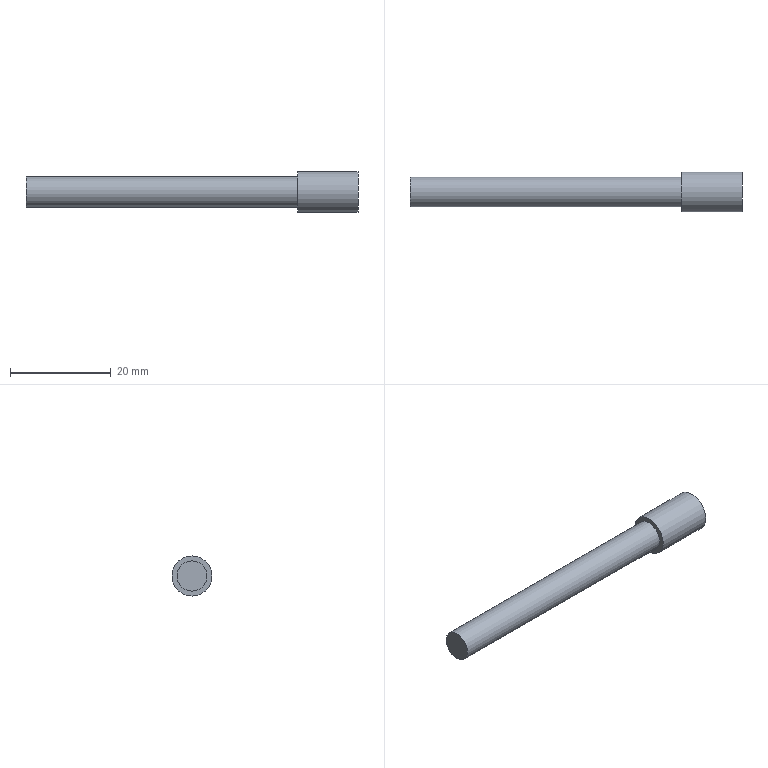Part | NX | features solid 2 | 1 solid | 5 faces | box 66 x 8 x 8 mm | volume 2130 mm3 | plane 3 | cylinder 2 | commonest cylinder face diameters 6 x1 8 x1
STEP:
#1=CARTESIAN_POINT('',(-71.,72.,-26.));
#2=VERTEX_POINT('',#1);
#3=CARTESIAN_POINT('',(-71.,72.,-23.));
#4=DIRECTION('',(-1.,0.,0.));
#5=DIRECTION('',(0.,0.,-1.));
#6=AXIS2_PLACEMENT_3D('',#3,#4,#5);
#7=CIRCLE('',#6,3.);
#8=EDGE_CURVE('',#2,#2,#7,.T.);
#9=ORIENTED_EDGE('',*,*,#8,.F.);
#10=EDGE_LOOP('',(#9));
#11=FACE_BOUND('',#10,.T.);
#12=CARTESIAN_POINT('',(-17.,72.,-20.));
#13=VERTEX_POINT('',#12);
#14=CARTESIAN_POINT('',(-17.,72.,-23.));
#15=DIRECTION('',(-1.,0.,0.));
#16=DIRECTION('',(0.,0.,1.));
#17=AXIS2_PLACEMENT_3D('',#14,#15,#16);
#18=CIRCLE('',#17,3.);
#19=EDGE_CURVE('',#13,#13,#18,.T.);
#20=ORIENTED_EDGE('',*,*,#19,.T.);
#21=EDGE_LOOP('',(#20));
#22=FACE_BOUND('',#21,.T.);
#23=CARTESIAN_POINT('',(-125.,72.,-23.));
#24=DIRECTION('',(1.,0.,0.));
#25=DIRECTION('',(0.,0.,1.));
#26=AXIS2_PLACEMENT_3D('',#23,#24,#25);
#27=CYLINDRICAL_SURFACE('',#26,3.);
#28=ADVANCED_FACE('',(#11,#22),#27,.T.);
#29=ORIENTED_EDGE('',*,*,#8,.T.);
#30=EDGE_LOOP('',(#29));
#31=FACE_BOUND('',#30,.T.);
#32=CARTESIAN_POINT('',(-71.,72.,-23.));
#33=DIRECTION('',(-1.,0.,0.));
#34=DIRECTION('',(0.,0.,-1.));
#35=AXIS2_PLACEMENT_3D('',#32,#33,#34);
#36=PLANE('',#35);
#37=ADVANCED_FACE('',(#31),#36,.T.);
#38=CARTESIAN_POINT('',(-17.,72.,-19.));
#39=VERTEX_POINT('',#38);
#40=CARTESIAN_POINT('',(-17.,72.,-23.));
#41=DIRECTION('',(-1.,0.,0.));
#42=DIRECTION('',(0.,0.,1.));
#43=AXIS2_PLACEMENT_3D('',#40,#41,#42);
#44=CIRCLE('',#43,4.);
#45=EDGE_CURVE('',#39,#39,#44,.T.);
#46=ORIENTED_EDGE('',*,*,#45,.T.);
#47=EDGE_LOOP('',(#46));
#48=FACE_BOUND('',#47,.T.);
#49=ORIENTED_EDGE('',*,*,#19,.F.);
#50=EDGE_LOOP('',(#49));
#51=FACE_BOUND('',#50,.T.);
#52=CARTESIAN_POINT('',(-17.,72.,-23.));
#53=DIRECTION('',(1.,0.,0.));
#54=DIRECTION('',(0.,0.,1.));
#55=AXIS2_PLACEMENT_3D('',#52,#53,#54);
#56=PLANE('',#55);
#57=ADVANCED_FACE('',(#48,#51),#56,.F.);
#58=ORIENTED_EDGE('',*,*,#45,.F.);
#59=EDGE_LOOP('',(#58));
#60=FACE_BOUND('',#59,.T.);
#61=CARTESIAN_POINT('',(-5.,72.,-19.));
#62=VERTEX_POINT('',#61);
#63=CARTESIAN_POINT('',(-5.,72.,-23.));
#64=DIRECTION('',(-1.,0.,0.));
#65=DIRECTION('',(0.,0.,1.));
#66=AXIS2_PLACEMENT_3D('',#63,#64,#65);
#67=CIRCLE('',#66,4.);
#68=EDGE_CURVE('',#62,#62,#67,.T.);
#69=ORIENTED_EDGE('',*,*,#68,.T.);
#70=EDGE_LOOP('',(#69));
#71=FACE_BOUND('',#70,.T.);
#72=CARTESIAN_POINT('',(-17.,72.,-23.));
#73=DIRECTION('',(1.,0.,0.));
#74=DIRECTION('',(0.,0.,1.));
#75=AXIS2_PLACEMENT_3D('',#72,#73,#74);
#76=CYLINDRICAL_SURFACE('',#75,4.);
#77=ADVANCED_FACE('',(#60,#71),#76,.T.);
#78=ORIENTED_EDGE('',*,*,#68,.F.);
#79=EDGE_LOOP('',(#78));
#80=FACE_BOUND('',#79,.T.);
#81=CARTESIAN_POINT('',(-5.,67.304,-33.));
#82=DIRECTION('',(1.,0.,0.));
#83=DIRECTION('',(0.,0.,1.));
#84=AXIS2_PLACEMENT_3D('',#81,#82,#83);
#85=PLANE('',#84);
#86=ADVANCED_FACE('',(#80),#85,.T.);
#87=CLOSED_SHELL('',(#28,#37,#57,#77,#86));
#88=MANIFOLD_SOLID_BREP('',#87);
#89=(LENGTH_UNIT()NAMED_UNIT(*)SI_UNIT(.MILLI.,.METRE.));
#90=UNCERTAINTY_MEASURE_WITH_UNIT(LENGTH_MEASURE(0.00001),#89,'','');
#91=(NAMED_UNIT(*)PLANE_ANGLE_UNIT()SI_UNIT($,.RADIAN.));
#92=(NAMED_UNIT(*)SI_UNIT($,.STERADIAN.)SOLID_ANGLE_UNIT());
#93=(GEOMETRIC_REPRESENTATION_CONTEXT(3)GLOBAL_UNCERTAINTY_ASSIGNED_CONTEXT((#90))GLOBAL_UNIT_ASSIGNED_CONTEXT((#89,#91,#92))REPRESENTATION_CONTEXT('',''));
#94=ADVANCED_BREP_SHAPE_REPRESENTATION('',(#88),#93);